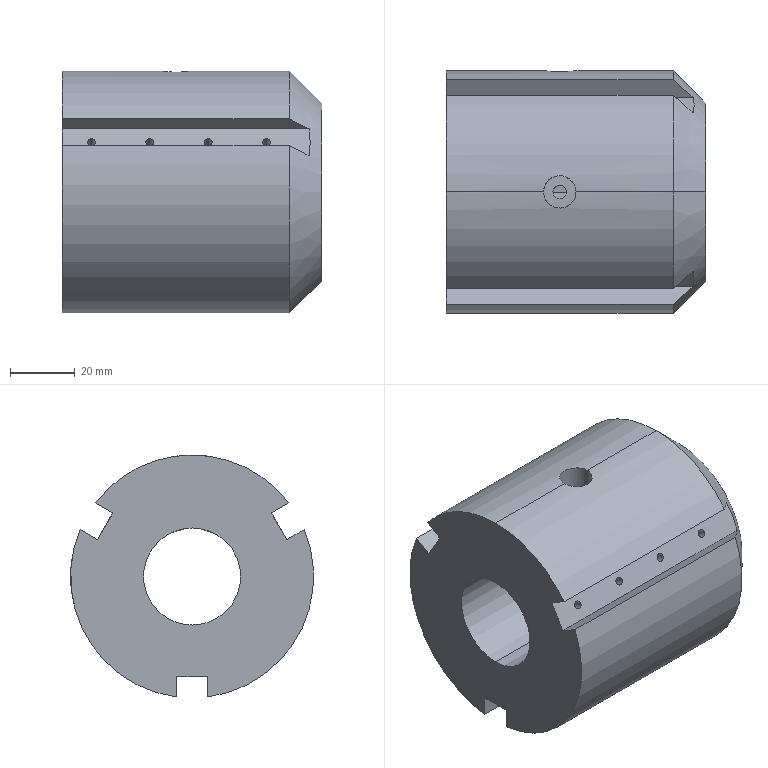Part | SolidWorks | features CirPattern 2, HoleWzd 2, ICE 2, Chamfer 1, Revolution 1 | 1 solid | 77 faces | box 80 x 75 x 74.698 mm | volume 269789 mm3 | cylinder 38 | cone 26 | plane 13 | commonest cylinder face diameters 2.5 x24 4.2 x4 10 x4 75 x4 30 x2